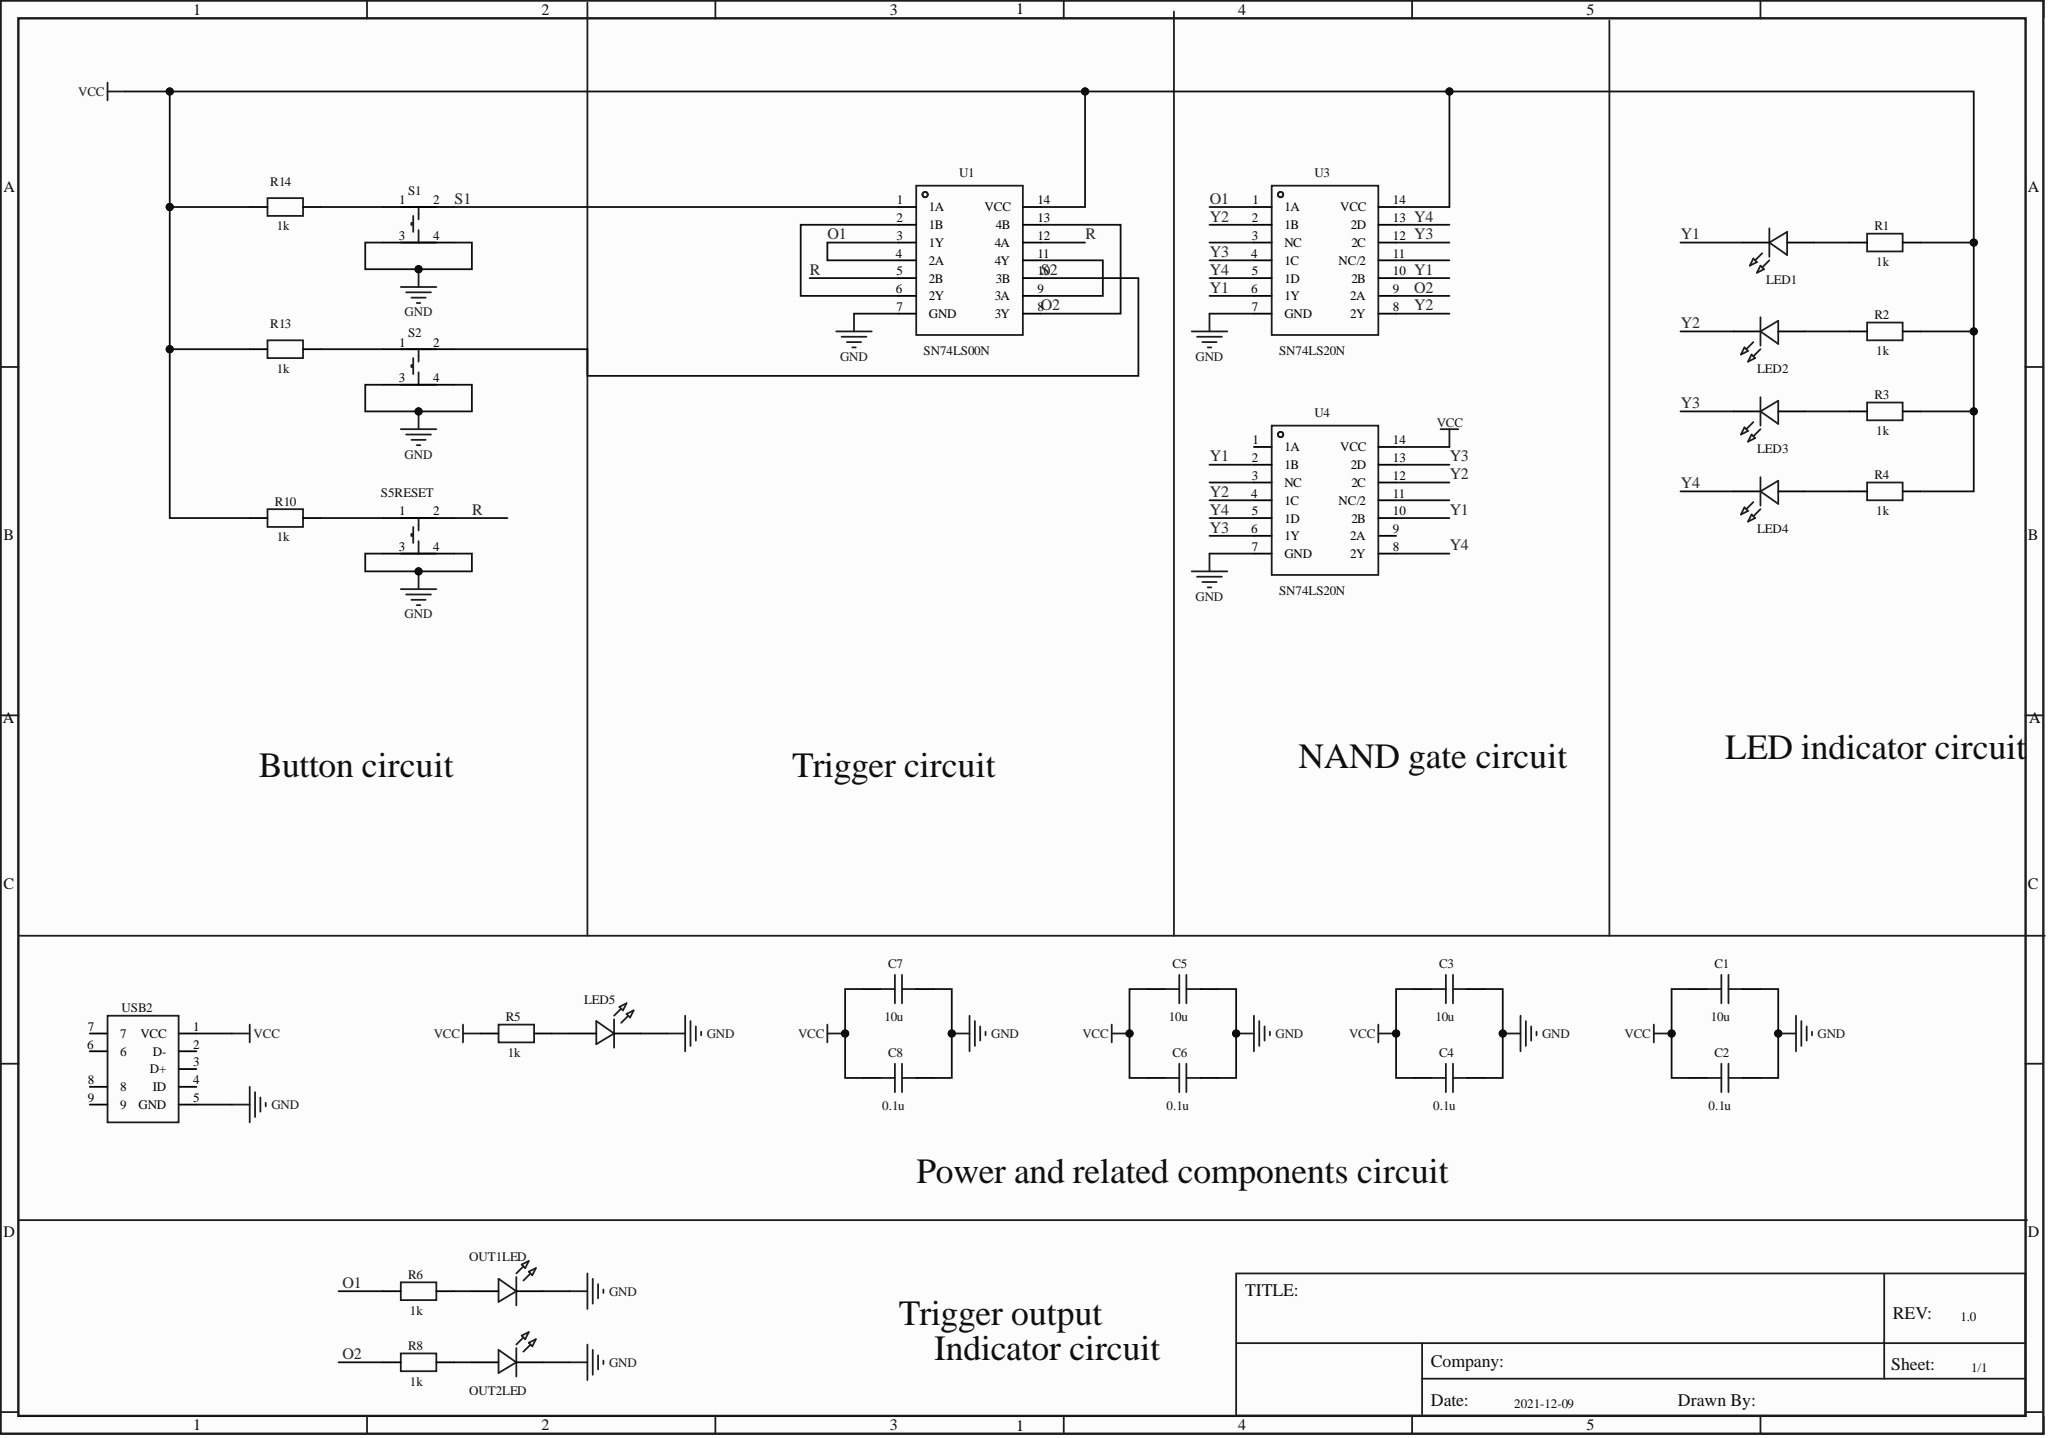Circuit board | Altium Designer | 32 parts | 23 nets
Bill of materials:
Comment,Description,Designator,Footprint,LibRef,Quantity
"10u","","C1, C3, C5, C7","C0805","10u","4"
"0.1u","","C2, C4, C6, C8","C0805","0.1u","4"
"LED-TH-5mm_R","","LED1, LED2, LED3, LED4, OUT1LED, OUT2LED","LED-TH_BD5.0_RED","333-2SURD/S530-A3","6"
"LED-TH-3mm_R","","LED5","LED-TH_BD3.0_RED","204-10SDRD/S530-A3-L","1"
"1k","","R1, R2, R3, R4, R5, R6, R8, R10, R13, R14","R0805","1k","10"
"TC-1157-B-A","","S1, S2, S5RESET","KEY-TH_4P-L6.4-W6.0-P4.50-LS7.3-TL","TC-1157-B-A","3"
"SN74LS00N","","U1","PDIP-14_L19.7-W6.6-P2.54-LS8.3-BL","SN74LS00N","1"
"SN74LS20N","","U3, U4","DIP-14_L19.0-W7.0-P2.54-LS7.6-BL","SN74LS20N","2"
"U-F-M5DD-W-2-SUS","","USB2","MICRO-USB-SMD_U-F-M5DD-W-2-SUS","U-F-M5DD-W-2-SUS","1"
Netlist (Protel format):
[
C1
C0805
10u



]
[
C2
C0805
0.1u



]
[
C3
C0805
10u



]
[
C4
C0805
0.1u



]
[
C5
C0805
10u



]
[
C6
C0805
0.1u



]
[
C7
C0805
10u



]
[
C8
C0805
0.1u



]
[
LED1
LED-TH_BD5.0_RED
LED-TH-5mm_R



]
[
LED2
LED-TH_BD5.0_RED
LED-TH-5mm_R



]
[
LED3
LED-TH_BD5.0_RED
LED-TH-5mm_R



]
[
LED4
LED-TH_BD5.0_RED
LED-TH-5mm_R



]
[
LED5
LED-TH_BD3.0_RED
LED-TH-3mm_R



]
[
OUT1LED
LED-TH_BD5.0_RED
LED-TH-5mm_R



]
[
OUT2LED
LED-TH_BD5.0_RED
LED-TH-5mm_R



]
[
R1
R0805
1k



]
[
R2
R0805
1k



]
[
R3
R0805
1k



]
[
R4
R0805
1k



]
[
R5
R0805
1k



]
[
R6
R0805
1k



]
[
R8
R0805
1k



]
[
R10
R0805
1k



]
[
R13
R0805
1k



]
[
R14
R0805
1k



]
[
S1
KEY-TH_4P-L6.4-W6.0-P4.50-LS7.3-TL
TC-1157-B-A



]
[
S2
KEY-TH_4P-L6.4-W6.0-P4.50-LS7.3-TL
TC-1157-B-A



]
[
S5RESET
KEY-TH_4P-L6.4-W6.0-P4.50-LS7.3-TL
TC-1157-B-A



]
[
U1
PDIP-14_L19.7-W6.6-P2.54-LS8.3-BL
SN74LS00N



]
[
U3
DIP-14_L19.0-W7.0-P2.54-LS7.6-BL
SN74LS20N



]
[
U4
DIP-14_L19.0-W7.0-P2.54-LS7.6-BL
SN74LS20N



]
[
USB2
MICRO-USB-SMD_U-F-M5DD-W-2-SUS
U-F-M5DD-W-2-SUS



]
(
Y4
LED4-2
U3-5
U3-13
U4-5
U4-8
)
(
Y3
LED3-2
U3-4
U3-12
U4-6
U4-13
)
(
Y2
LED2-2
U3-2
U3-8
U4-4
U4-12
)
(
Y1
LED1-2
U3-6
U3-10
U4-2
U4-10
)
(
VCC
C1-1
C2-1
C3-1
C4-1
C5-1
C6-1
C7-1
C8-1
R1-2
R2-2
R3-2
R4-2
R5-1
R10-1
R13-1
R14-1
U1-14
U3-14
U4-14
USB2-1
)
(
S2
S2-2
U1-10
)
(
S1
S1-2
U1-1
)
(
R
S5RESET-2
U1-5
U1-12
)
(
O2
R8-1
U1-8
U1-13
U3-9
)
(
O1
R6-1
U1-3
U1-4
U3-1
)
(
NetU1_9
U1-9
U1-11
)
(
NetU1_2
U1-2
U1-6
)
(
NetR14_2
R14-2
S1-1
)
(
NetR13_2
R13-2
S2-1
)
(
NetR10_2
R10-2
S5RESET-1
)
(
NetOUT2LED_1
OUT2LED-1
R8-2
)
(
NetOUT1LED_1
OUT1LED-1
R6-2
)
(
NetLED5_1
LED5-1
R5-2
)
(
NetLED4_1
LED4-1
R4-1
)
(
NetLED3_1
LED3-1
R3-1
)
(
NetLED2_1
LED2-1
R2-1
)
(
NetLED1_1
LED1-1
R1-1
)
(
GND
C1-2
C2-2
C3-2
C4-2
C5-2
C6-2
C7-2
C8-2
LED5-2
OUT1LED-2
OUT2LED-2
S1-3
S1-4
S2-3
S2-4
S5RESET-3
S5RESET-4
U1-7
U3-7
U4-7
USB2-5
)